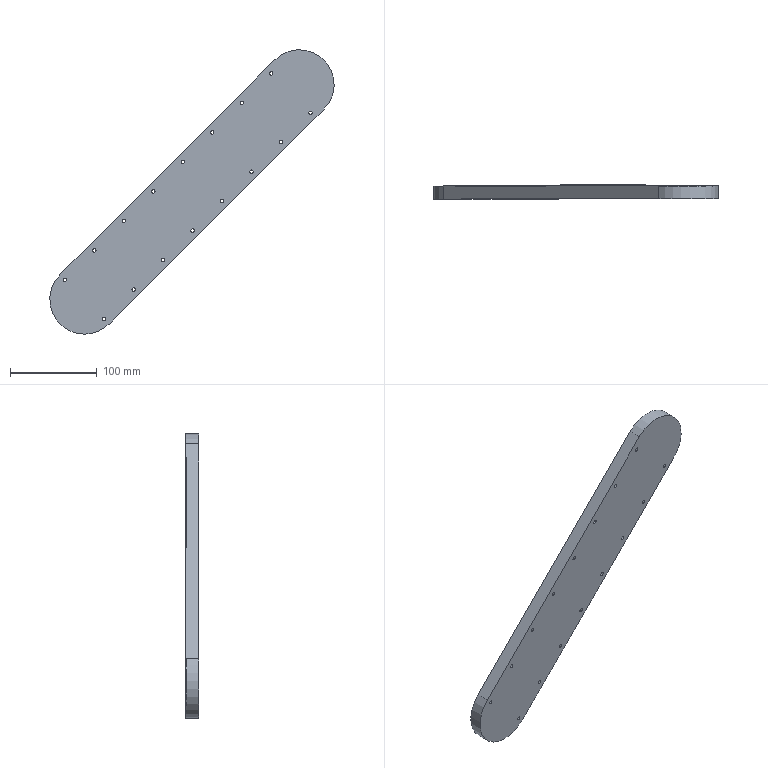Part | SolidWorks | features ICE 3, Emboss 1, Extrusion 1, LPattern 1, MirrorPattern 1 | 1 solid | 309 faces | box 327.487 x 16 x 327.487 mm | volume 460753 mm3 | spline 126 | plane 113 | cylinder 70 | commonest cylinder face diameters 4 x32 8 x32 78 x3 80 x3